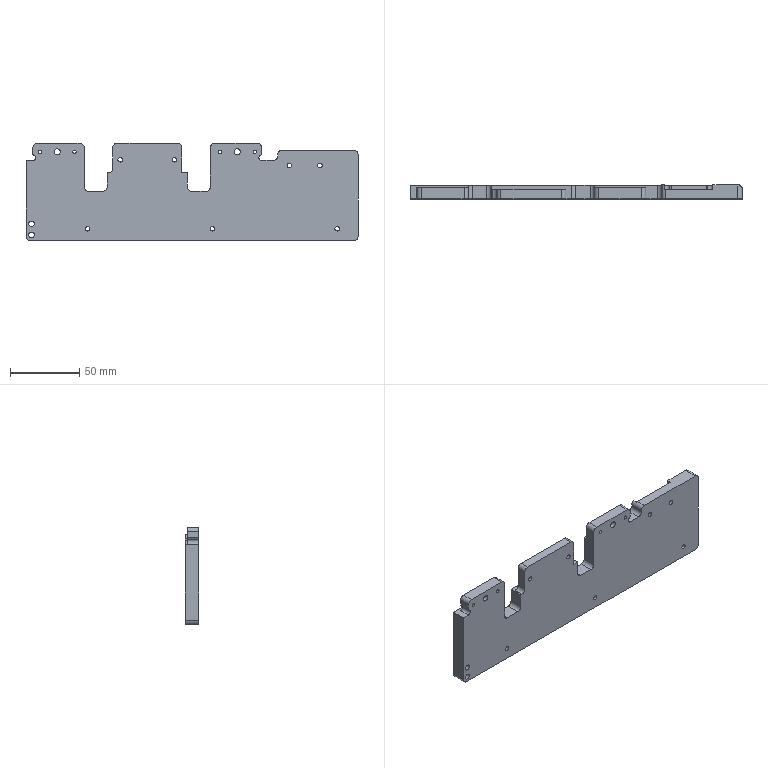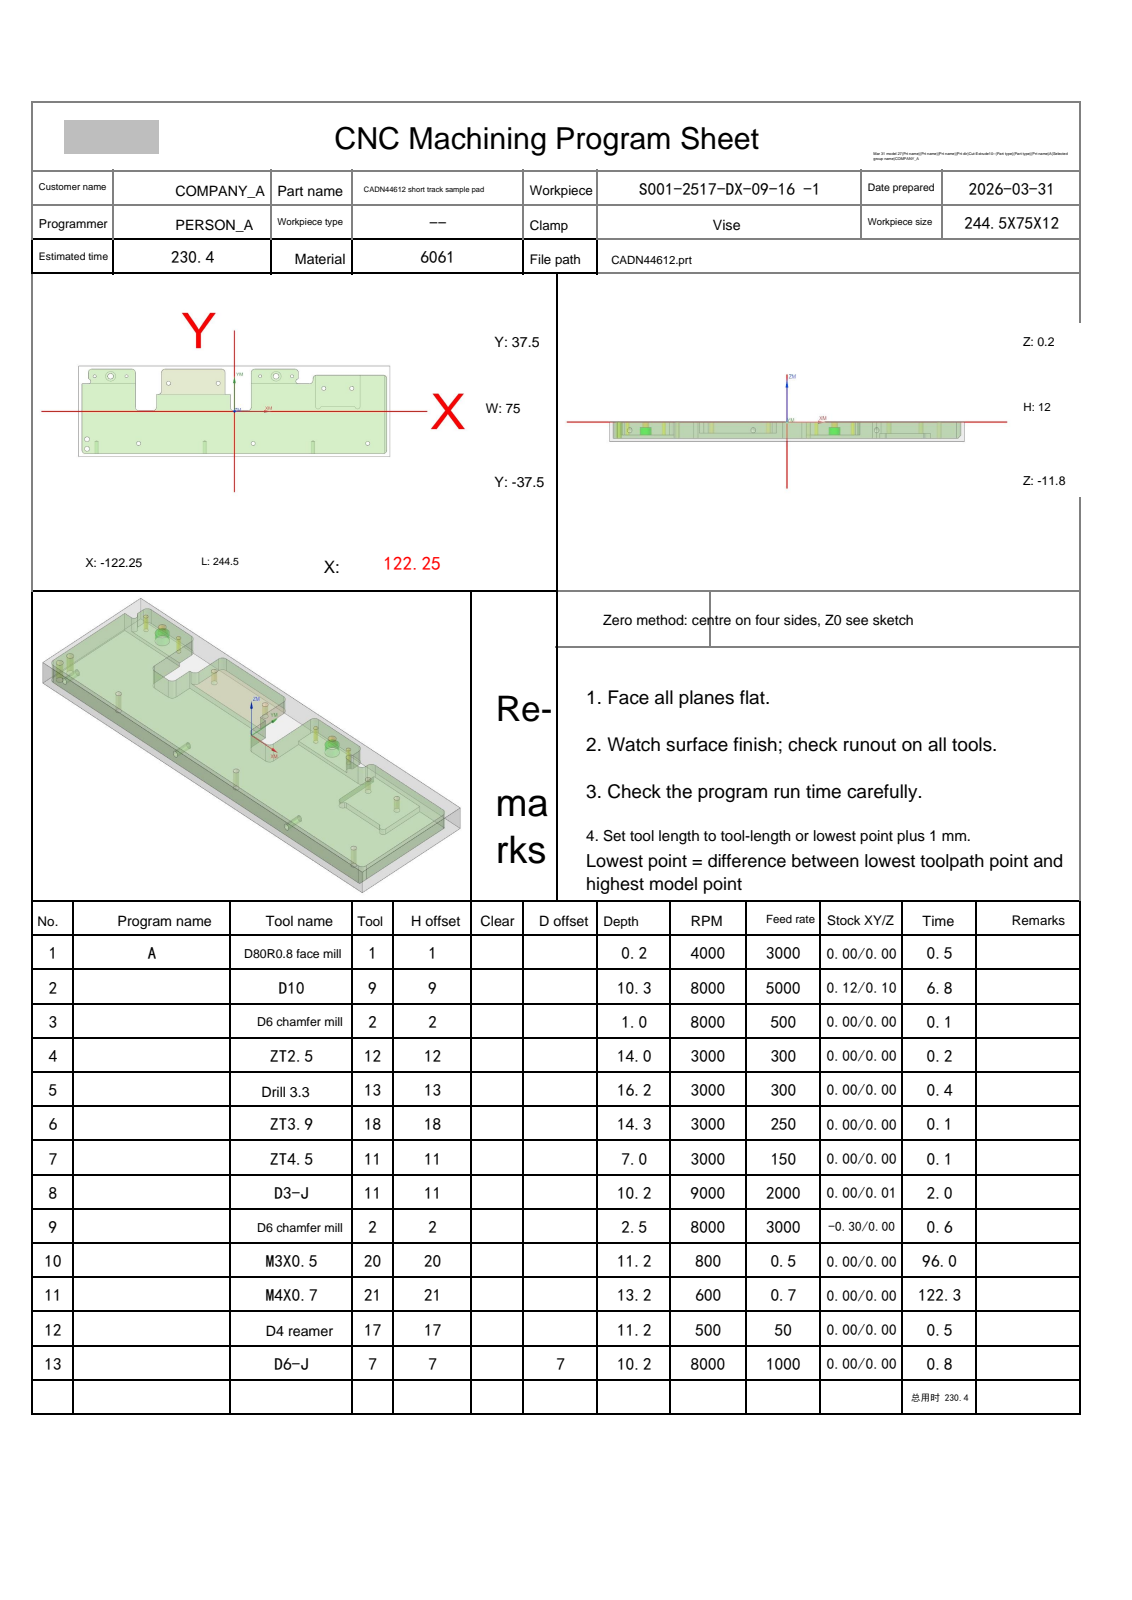NC program | NX | posted by the shop | part box 239.5 x 10 x 70 mm
Lines 2414 to 3395 of 10745:
N8 T11 M06
(D3-J  D=3. R=0. H=11 ce=0.00 di=0.01)
G00 G90 G54 X-120.212 Y24.718 M03 S9000
G43 H11 Z20.
M08
Z.157
G01 X-120.211 Y24.713 Z.093 F1600.
X-120.207 Y24.699 Z.035
X-120.201 Y24.677 Z-.018
X-120.193 Y24.649 Z-.065
X-120.182 Y24.616 Z-.107
X-120.168 Y24.579 Z-.143
X-120.152 Y24.539 Z-.175
X-120.133 Y24.499 Z-.203
X-120.111 Y24.459 Z-.226
X-120.087 Y24.42 Z-.245
X-120.059 Y24.384 Z-.261
X-120.029 Y24.352 Z-.273
X-119.995 Y24.326 Z-.282
X-119.958 Y24.307 Z-.288
X-119.918 Y24.296 Z-.292
X-119.875 Y24.295 Z-.293
X-119.75 Y24.3 F2000.
X-114.75
G03 X-114.25 Y24.8 I0.0 J.5
X-114.583 Y25.271 I-.5 J0.0
G02 X-116.25 Y27.628 I.833 J2.357
G01 Y27.973
X-116.266 Y28.001 Z-.294
X-116.312 Y28.005 Z-.296
X-116.384 Y27.986 Z-.3
X-116.48 Y27.947 Z-.306
X-116.596 Y27.889 Z-.312
X-116.729 Y27.815 Z-.32
X-117.029 Y27.625 Z-.339
X-117.224 Y27.491 Z-.351
X-117.539 Y27.259 Z-.372
X-117.999 Y26.878 Z-.405
X-118.437 Y26.464 Z-.439
X-118.844 Y26.024 Z-.473
X-119.214 Y25.564 Z-.506
X-119.436 Y25.25 Z-.527
X-119.562 Y25.056 Z-.539
X-119.739 Y24.759 Z-.558
X-119.808 Y24.627 Z-.565
X-119.86 Y24.513 Z-.572
X-119.895 Y24.42 Z-.578
X-119.91 Y24.35 Z-.582
X-119.904 Y24.307 Z-.584
X-119.875 Y24.295 Z-.585
X-119.75 Y24.3
X-114.75
G03 X-114.25 Y24.8 I0.0 J.5
X-114.583 Y25.271 I-.5 J0.0
G02 X-116.25 Y27.628 I.833 J2.357
G01 Y27.973
X-116.266 Y28.001 Z-.586
X-116.312 Y28.005 Z-.589
X-116.384 Y27.986 Z-.593
X-116.48 Y27.947 Z-.598
X-116.596 Y27.889 Z-.605
X-116.729 Y27.815 Z-.613
X-117.029 Y27.625 Z-.631
X-117.224 Y27.491 Z-.644
X-117.539 Y27.259 Z-.665
X-117.999 Y26.878 Z-.698
X-118.437 Y26.464 Z-.732
X-118.844 Y26.024 Z-.766
X-119.214 Y25.564 Z-.799
X-119.436 Y25.25 Z-.819
X-119.562 Y25.056 Z-.832
X-119.739 Y24.759 Z-.85
X-119.808 Y24.627 Z-.858
X-119.86 Y24.513 Z-.865
X-119.895 Y24.42 Z-.87
X-119.91 Y24.35 Z-.874
X-119.904 Y24.307 Z-.877
X-119.875 Y24.295 Z-.878
X-119.75 Y24.3
X-114.75
G03 X-114.25 Y24.8 I0.0 J.5
X-114.583 Y25.271 I-.5 J0.0
G02 X-116.25 Y27.628 I.833 J2.357
G01 Y27.973
X-116.266 Y28.001 Z-.879
X-116.312 Y28.005 Z-.881
X-116.384 Y27.986 Z-.885
X-116.48 Y27.947 Z-.891
X-116.596 Y27.889 Z-.898
X-116.729 Y27.815 Z-.906
X-117.029 Y27.625 Z-.924
X-117.224 Y27.491 Z-.936
X-117.539 Y27.259 Z-.957
X-117.999 Y26.878 Z-.99
X-118.437 Y26.464 Z-1.024
X-118.844 Y26.024 Z-1.058
X-119.214 Y25.564 Z-1.091
X-119.436 Y25.25 Z-1.112
X-119.562 Y25.056 Z-1.124
X-119.739 Y24.759 Z-1.143
X-119.808 Y24.627 Z-1.151
X-119.86 Y24.513 Z-1.158
X-119.895 Y24.42 Z-1.163
X-119.91 Y24.35 Z-1.167
X-119.904 Y24.307 Z-1.17
X-119.875 Y24.295 Z-1.171
X-119.75 Y24.3
X-114.75
G03 X-114.25 Y24.8 I0.0 J.5
X-114.583 Y25.271 I-.5 J0.0
G02 X-116.25 Y27.628 I.833 J2.357
G01 Y27.973
X-116.266 Y28.001
X-116.312 Y28.005 Z-1.174
X-116.384 Y27.986 Z-1.178
X-116.48 Y27.947 Z-1.184
X-116.596 Y27.889 Z-1.19
X-116.729 Y27.815 Z-1.198
X-117.029 Y27.625 Z-1.217
X-117.224 Y27.491 Z-1.229
X-117.539 Y27.259 Z-1.25
X-117.999 Y26.878 Z-1.283
X-118.437 Y26.464 Z-1.317
X-118.844 Y26.024 Z-1.351
X-119.214 Y25.564 Z-1.384
X-119.436 Y25.25 Z-1.405
X-119.562 Y25.056 Z-1.417
X-119.739 Y24.759 Z-1.436
X-119.808 Y24.627 Z-1.443
X-119.86 Y24.513 Z-1.45
X-119.895 Y24.42 Z-1.456
X-119.91 Y24.35 Z-1.46
X-119.904 Y24.307 Z-1.462
X-119.875 Y24.295 Z-1.463
X-119.75 Y24.3
X-114.75
G03 X-114.25 Y24.8 I0.0 J.5
X-114.583 Y25.271 I-.5 J0.0
G02 X-116.25 Y27.628 I.833 J2.357
G01 Y27.973
X-116.266 Y28.001 Z-1.464
X-116.312 Y28.005 Z-1.467
X-116.384 Y27.986 Z-1.471
X-116.48 Y27.947 Z-1.476
X-116.596 Y27.889 Z-1.483
X-116.729 Y27.815 Z-1.491
X-117.029 Y27.625 Z-1.509
X-117.224 Y27.491 Z-1.522
X-117.539 Y27.259 Z-1.542
X-117.999 Y26.878 Z-1.575
X-118.437 Y26.464 Z-1.61
X-118.844 Y26.024 Z-1.644
X-119.214 Y25.564 Z-1.677
X-119.436 Y25.25 Z-1.697
X-119.562 Y25.056 Z-1.71
X-119.739 Y24.759 Z-1.728
X-119.808 Y24.627 Z-1.736
X-119.86 Y24.513 Z-1.743
X-119.895 Y24.42 Z-1.748
X-119.91 Y24.35 Z-1.752
X-119.904 Y24.307 Z-1.755
X-119.875 Y24.295 Z-1.756
X-119.75 Y24.3
X-114.75
G03 X-114.25 Y24.8 I0.0 J.5
X-114.583 Y25.271 I-.5 J0.0
G02 X-116.25 Y27.628 I.833 J2.357
G01 Y27.973
X-116.266 Y28.001 Z-1.757
X-116.312 Y28.005 Z-1.759
X-116.384 Y27.986 Z-1.763
X-116.48 Y27.947 Z-1.769
X-116.596 Y27.889 Z-1.776
X-116.729 Y27.815 Z-1.784
X-117.029 Y27.625 Z-1.802
X-117.224 Y27.491 Z-1.814
X-117.539 Y27.259 Z-1.835
X-117.999 Y26.878 Z-1.868
X-118.437 Y26.464 Z-1.902
X-118.844 Y26.024 Z-1.936
X-119.214 Y25.564 Z-1.969
X-119.436 Y25.25 Z-1.99
X-119.562 Y25.056 Z-2.002
X-119.739 Y24.759 Z-2.021
X-119.808 Y24.627 Z-2.029
X-119.86 Y24.513 Z-2.035
X-119.895 Y24.42 Z-2.041
X-119.91 Y24.35 Z-2.045
X-119.904 Y24.307 Z-2.048
X-119.875 Y24.295 Z-2.049
X-119.75 Y24.3
X-114.75
G03 X-114.25 Y24.8 I0.0 J.5
X-114.583 Y25.271 I-.5 J0.0
G02 X-116.25 Y27.628 I.833 J2.357
G01 Y27.973
X-116.266 Y28.001
X-116.312 Y28.005 Z-2.052
X-116.384 Y27.986 Z-2.056
X-116.48 Y27.947 Z-2.062
X-116.596 Y27.889 Z-2.068
X-116.729 Y27.815 Z-2.076
X-117.029 Y27.625 Z-2.095
X-117.224 Y27.491 Z-2.107
X-117.539 Y27.259 Z-2.128
X-117.999 Y26.878 Z-2.161
X-118.437 Y26.464 Z-2.195
X-118.844 Y26.024 Z-2.229
X-119.214 Y25.564 Z-2.262
X-119.436 Y25.25 Z-2.283
X-119.562 Y25.056 Z-2.295
X-119.739 Y24.759 Z-2.313
X-119.808 Y24.627 Z-2.321
X-119.86 Y24.513 Z-2.328
X-119.895 Y24.42 Z-2.334
X-119.91 Y24.35 Z-2.338
X-119.904 Y24.307 Z-2.34
X-119.875 Y24.295 Z-2.341
X-119.75 Y24.3
X-114.75
G03 X-114.25 Y24.8 I0.0 J.5
X-114.583 Y25.271 I-.5 J0.0
G02 X-116.25 Y27.628 I.833 J2.357
G01 Y27.973
X-116.266 Y28.001 Z-2.342
X-116.312 Y28.005 Z-2.345
X-116.384 Y27.986 Z-2.349
X-116.48 Y27.947 Z-2.354
X-116.596 Y27.889 Z-2.361
X-116.729 Y27.815 Z-2.369
X-117.029 Y27.625 Z-2.387
X-117.224 Y27.491 Z-2.4
X-117.539 Y27.259 Z-2.42
X-117.999 Y26.878 Z-2.453
X-118.437 Y26.464 Z-2.488
X-118.844 Y26.024 Z-2.522
X-119.214 Y25.564 Z-2.555
X-119.436 Y25.25 Z-2.575
X-119.562 Y25.056 Z-2.588
X-119.739 Y24.759 Z-2.606
X-119.808 Y24.627 Z-2.614
X-119.86 Y24.513 Z-2.621
X-119.895 Y24.42 Z-2.626
X-119.91 Y24.35 Z-2.63
X-119.904 Y24.307 Z-2.633
X-119.875 Y24.295 Z-2.634
X-119.75 Y24.3
X-114.75
G03 X-114.25 Y24.8 I0.0 J.5
X-114.583 Y25.271 I-.5 J0.0
G02 X-116.25 Y27.628 I.833 J2.357
G01 Y27.973
X-116.266 Y28.001 Z-2.635
X-116.312 Y28.005 Z-2.637
X-116.384 Y27.986 Z-2.641
X-116.48 Y27.947 Z-2.647
X-116.596 Y27.889 Z-2.654
X-116.729 Y27.815 Z-2.662
X-117.029 Y27.625 Z-2.68
X-117.224 Y27.491 Z-2.692
X-117.539 Y27.259 Z-2.713
X-117.999 Y26.878 Z-2.746
X-118.437 Y26.464 Z-2.78
X-118.844 Y26.024 Z-2.814
X-119.214 Y25.564 Z-2.847
X-119.436 Y25.25 Z-2.868
X-119.562 Y25.056 Z-2.88
X-119.739 Y24.759 Z-2.899
X-119.808 Y24.627 Z-2.907
X-119.86 Y24.513 Z-2.913
X-119.895 Y24.42 Z-2.919
X-119.91 Y24.35 Z-2.923
X-119.904 Y24.307 Z-2.926
X-119.875 Y24.295
X-119.75 Y24.3
X-114.75
G03 X-114.25 Y24.8 I0.0 J.5
X-114.583 Y25.271 I-.5 J0.0
G02 X-116.25 Y27.628 I.833 J2.357
G01 Y27.973
X-116.266 Y28.001 Z-2.927
X-116.312 Y28.005 Z-2.93
X-116.384 Y27.986 Z-2.934
X-116.48 Y27.947 Z-2.94
X-116.596 Y27.889 Z-2.946
X-116.729 Y27.815 Z-2.954
X-117.029 Y27.625 Z-2.973
X-117.224 Y27.491 Z-2.985
X-117.539 Y27.259 Z-3.006
X-117.999 Y26.878 Z-3.039
X-118.437 Y26.464 Z-3.073
X-118.844 Y26.024 Z-3.107
X-119.214 Y25.564 Z-3.14
X-119.436 Y25.25 Z-3.161
X-119.562 Y25.056 Z-3.173
X-119.739 Y24.759 Z-3.191
X-119.808 Y24.627 Z-3.199
X-119.86 Y24.513 Z-3.206
X-119.895 Y24.42 Z-3.212
X-119.91 Y24.35 Z-3.216
X-119.904 Y24.307 Z-3.218
X-119.875 Y24.295 Z-3.219
X-119.75 Y24.3
X-114.75
G03 X-114.25 Y24.8 I0.0 J.5
X-114.583 Y25.271 I-.5 J0.0
G02 X-116.25 Y27.628 I.833 J2.357
G01 Y27.973
X-116.266 Y28.001 Z-3.22
X-116.312 Y28.005 Z-3.223
X-116.384 Y27.986 Z-3.227
X-116.48 Y27.947 Z-3.232
X-116.596 Y27.889 Z-3.239
X-116.729 Y27.815 Z-3.247
X-117.029 Y27.625 Z-3.265
X-117.224 Y27.491 Z-3.278
X-117.539 Y27.259 Z-3.298
X-117.999 Y26.878 Z-3.331
X-118.437 Y26.464 Z-3.365
X-118.844 Y26.024 Z-3.4
X-119.214 Y25.564 Z-3.433
X-119.436 Y25.25 Z-3.453
X-119.562 Y25.056 Z-3.466
X-119.739 Y24.759 Z-3.484
X-119.808 Y24.627 Z-3.492
X-119.86 Y24.513 Z-3.499
X-119.895 Y24.42 Z-3.504
X-119.91 Y24.35 Z-3.508
X-119.904 Y24.307 Z-3.511
X-119.875 Y24.295 Z-3.512
X-119.75 Y24.3
X-114.75
G03 X-114.25 Y24.8 I0.0 J.5
X-114.583 Y25.271 I-.5 J0.0
G02 X-116.25 Y27.628 I.833 J2.357
G01 Y27.973
X-116.266 Y28.001 Z-3.513
X-116.312 Y28.005 Z-3.515
X-116.384 Y27.986 Z-3.519
X-116.48 Y27.947 Z-3.525
X-116.596 Y27.889 Z-3.532
X-116.729 Y27.815 Z-3.539
X-117.029 Y27.625 Z-3.558
X-117.224 Y27.491 Z-3.57
X-117.539 Y27.259 Z-3.591
X-117.999 Y26.878 Z-3.624
X-118.437 Y26.464 Z-3.658
X-118.844 Y26.024 Z-3.692
X-119.214 Y25.564 Z-3.725
X-119.436 Y25.25 Z-3.746
X-119.562 Y25.056 Z-3.758
X-119.739 Y24.759 Z-3.777
X-119.808 Y24.627 Z-3.785
X-119.86 Y24.513 Z-3.791
X-119.895 Y24.42 Z-3.797
X-119.91 Y24.35 Z-3.801
X-119.904 Y24.307 Z-3.804
X-119.875 Y24.295
X-119.75 Y24.3
X-114.75
G03 X-114.25 Y24.8 I0.0 J.5
X-114.583 Y25.271 I-.5 J0.0
G02 X-116.25 Y27.628 I.833 J2.357
G01 Y27.973
X-116.266 Y28.001 Z-3.805
X-116.312 Y28.005 Z-3.808
X-116.384 Y27.986 Z-3.812
X-116.48 Y27.947 Z-3.817
X-116.596 Y27.889 Z-3.824
X-116.729 Y27.815 Z-3.832
X-117.029 Y27.625 Z-3.85
X-117.224 Y27.491 Z-3.863
X-117.539 Y27.259 Z-3.884
X-117.999 Y26.878 Z-3.917
X-118.437 Y26.464 Z-3.951
X-118.844 Y26.024 Z-3.985
X-119.214 Y25.564 Z-4.018
X-119.436 Y25.25 Z-4.039
X-119.562 Y25.056 Z-4.051
X-119.739 Y24.759 Z-4.069
X-119.808 Y24.627 Z-4.077
X-119.86 Y24.513 Z-4.084
X-119.895 Y24.42 Z-4.09
X-119.91 Y24.35 Z-4.094
X-119.904 Y24.307 Z-4.096
X-119.875 Y24.295 Z-4.097
X-119.75 Y24.3
X-114.75
G03 X-114.25 Y24.8 I0.0 J.5
X-114.583 Y25.271 I-.5 J0.0
G02 X-116.25 Y27.628 I.833 J2.357
G01 Y27.973
X-116.266 Y28.001 Z-4.098
X-116.312 Y28.005 Z-4.101
X-116.384 Y27.986 Z-4.105
X-116.48 Y27.947 Z-4.11
X-116.596 Y27.889 Z-4.117
X-116.729 Y27.815 Z-4.125
X-117.029 Y27.625 Z-4.143
X-117.224 Y27.491 Z-4.155
X-117.539 Y27.259 Z-4.176
X-117.999 Y26.878 Z-4.209
X-118.437 Y26.464 Z-4.243
X-118.844 Y26.024 Z-4.277
X-119.214 Y25.564 Z-4.31
X-119.436 Y25.25 Z-4.331
X-119.562 Y25.056 Z-4.344
X-119.739 Y24.759 Z-4.362
X-119.808 Y24.627 Z-4.37
X-119.86 Y24.513 Z-4.377
X-119.895 Y24.42 Z-4.382
X-119.91 Y24.35 Z-4.386
X-119.904 Y24.307 Z-4.389
X-119.875 Y24.295 Z-4.39
X-119.75 Y24.3
X-114.75
G03 X-114.25 Y24.8 I0.0 J.5
X-114.583 Y25.271 I-.5 J0.0
G02 X-116.25 Y27.628 I.833 J2.357
G01 Y27.973
X-116.266 Y28.001 Z-4.391
X-116.312 Y28.005 Z-4.393
X-116.384 Y27.986 Z-4.397
X-116.48 Y27.947 Z-4.403
X-116.596 Y27.889 Z-4.41
X-116.729 Y27.815 Z-4.417
X-117.029 Y27.625 Z-4.436
X-117.224 Y27.491 Z-4.448
X-117.539 Y27.259 Z-4.469
X-117.999 Y26.878 Z-4.502
X-118.437 Y26.464 Z-4.536
X-118.844 Y26.024 Z-4.57
X-119.214 Y25.564 Z-4.603
X-119.436 Y25.25 Z-4.624
X-119.562 Y25.056 Z-4.636
X-119.739 Y24.759 Z-4.655
X-119.808 Y24.627 Z-4.663
X-119.86 Y24.513 Z-4.669
X-119.895 Y24.42 Z-4.675
X-119.91 Y24.35 Z-4.679
X-119.904 Y24.307 Z-4.681
X-119.875 Y24.295 Z-4.682
X-119.75 Y24.3
X-114.75
G03 X-114.25 Y24.8 I0.0 J.5
X-114.583 Y25.271 I-.5 J0.0
G02 X-116.25 Y27.628 I.833 J2.357
G01 Y27.973
X-116.266 Y28.001 Z-4.683
X-116.312 Y28.005 Z-4.686
X-116.384 Y27.986 Z-4.69
X-116.48 Y27.947 Z-4.695
X-116.596 Y27.889 Z-4.702
X-116.729 Y27.815 Z-4.71
X-117.029 Y27.625 Z-4.728
X-117.224 Y27.491 Z-4.741
X-117.539 Y27.259 Z-4.762
X-117.999 Y26.878 Z-4.795
X-118.437 Y26.464 Z-4.829
X-118.844 Y26.024 Z-4.863
X-119.214 Y25.564 Z-4.896
X-119.436 Y25.25 Z-4.917
X-119.562 Y25.056 Z-4.929
X-119.739 Y24.759 Z-4.947
X-119.808 Y24.627 Z-4.955
X-119.86 Y24.513 Z-4.962
X-119.895 Y24.42 Z-4.967
X-119.91 Y24.35 Z-4.972
X-119.904 Y24.307 Z-4.974
X-119.875 Y24.295 Z-4.975
X-119.75 Y24.3
X-114.75
G03 X-114.25 Y24.8 I0.0 J.5
X-114.583 Y25.271 I-.5 J0.0
G02 X-116.25 Y27.628 I.833 J2.357
G01 Y27.973
X-116.266 Y28.001 Z-4.976
X-116.312 Y28.005 Z-4.978
X-116.384 Y27.986 Z-4.983
X-116.48 Y27.947 Z-4.988
X-116.596 Y27.889 Z-4.995
X-116.729 Y27.815 Z-5.003
X-117.029 Y27.625 Z-5.021
X-117.224 Y27.491 Z-5.033
X-117.539 Y27.259 Z-5.054
X-117.999 Y26.878 Z-5.087
X-118.437 Y26.464 Z-5.121
X-118.844 Y26.024 Z-5.155
X-119.214 Y25.564 Z-5.188
X-119.436 Y25.25 Z-5.209
X-119.562 Y25.056 Z-5.222
X-119.739 Y24.759 Z-5.24
X-119.808 Y24.627 Z-5.248
X-119.86 Y24.513 Z-5.255
X-119.895 Y24.42 Z-5.26
X-119.91 Y24.35 Z-5.264
X-119.904 Y24.307 Z-5.267
X-119.875 Y24.295 Z-5.268
X-119.75 Y24.3
X-114.75
G03 X-114.25 Y24.8 I0.0 J.5
X-114.583 Y25.271 I-.5 J0.0
G02 X-116.25 Y27.628 I.833 J2.357
G01 Y27.973
X-116.266 Y28.001 Z-5.269
X-116.312 Y28.005 Z-5.271
X-116.384 Y27.986 Z-5.275
X-116.48 Y27.947 Z-5.281
X-116.596 Y27.889 Z-5.287
X-116.729 Y27.815 Z-5.295
X-117.029 Y27.625 Z-5.314
X-117.224 Y27.491 Z-5.326
X-117.539 Y27.259 Z-5.347
X-117.999 Y26.878 Z-5.38
X-118.437 Y26.464 Z-5.414
X-118.844 Y26.024 Z-5.448
X-119.214 Y25.564 Z-5.481
X-119.436 Y25.25 Z-5.502
X-119.562 Y25.056 Z-5.514
X-119.739 Y24.759 Z-5.533
X-119.808 Y24.627 Z-5.54
X-119.86 Y24.513 Z-5.547
X-119.895 Y24.42 Z-5.553
X-119.91 Y24.35 Z-5.557
X-119.904 Y24.307 Z-5.559
X-119.875 Y24.295 Z-5.56
X-119.75 Y24.3
X-114.75
G03 X-114.25 Y24.8 I0.0 J.5
X-114.583 Y25.271 I-.5 J0.0
G02 X-116.25 Y27.628 I.833 J2.357
G01 Y27.973
X-116.266 Y28.001 Z-5.561
X-116.312 Y28.005 Z-5.564
X-116.384 Y27.986 Z-5.568
X-116.48 Y27.947 Z-5.573
X-116.596 Y27.889 Z-5.58
X-116.729 Y27.815 Z-5.588
X-117.029 Y27.625 Z-5.606
X-117.224 Y27.491 Z-5.619
X-117.539 Y27.259 Z-5.64
X-117.999 Y26.878 Z-5.673
X-118.437 Y26.464 Z-5.707
X-118.844 Y26.024 Z-5.741
X-119.214 Y25.564 Z-5.774
X-119.436 Y25.25 Z-5.794
X-119.562 Y25.056 Z-5.807
X-119.739 Y24.759 Z-5.825
X-119.808 Y24.627 Z-5.833
X-119.86 Y24.513 Z-5.84
X-119.895 Y24.42 Z-5.845
X-119.91 Y24.35 Z-5.849
X-119.904 Y24.307 Z-5.852
X-119.875 Y24.295 Z-5.853
X-119.75 Y24.3
X-114.75
G03 X-114.25 Y24.8 I0.0 J.5
X-114.583 Y25.271 I-.5 J0.0
G02 X-116.25 Y27.628 I.833 J2.357
G01 Y27.973
X-116.266 Y28.001 Z-5.854
X-116.312 Y28.005 Z-5.856
X-116.384 Y27.986 Z-5.86
X-116.48 Y27.947 Z-5.866
X-116.596 Y27.889 Z-5.873
X-116.729 Y27.815 Z-5.881
X-117.029 Y27.625 Z-5.899
X-117.224 Y27.491 Z-5.911
X-117.539 Y27.259 Z-5.932
X-117.999 Y26.878 Z-5.965
X-118.437 Y26.464 Z-5.999
X-118.844 Y26.024 Z-6.033
X-119.214 Y25.564 Z-6.066
X-119.436 Y25.25 Z-6.087
X-119.562 Y25.056 Z-6.099
X-119.739 Y24.759 Z-6.118
X-119.808 Y24.627 Z-6.126
X-119.86 Y24.513 Z-6.133
X-119.895 Y24.42 Z-6.138
X-119.91 Y24.35 Z-6.142
X-119.904 Y24.307 Z-6.145
X-119.875 Y24.295 Z-6.146
X-119.75 Y24.3
X-114.75
G03 X-114.25 Y24.8 I0.0 J.5
X-114.583 Y25.271 I-.5 J0.0
G02 X-116.25 Y27.628 I.833 J2.357
G01 Y27.973
X-116.266 Y28.001
X-116.312 Y28.005 Z-6.149
X-116.384 Y27.986 Z-6.153
X-116.48 Y27.947 Z-6.159
X-116.596 Y27.889 Z-6.165
X-116.729 Y27.815 Z-6.173
X-117.029 Y27.625 Z-6.192
X-117.224 Y27.491 Z-6.204
X-117.539 Y27.259 Z-6.225
X-117.999 Y26.878 Z-6.258
X-118.437 Y26.464 Z-6.292
X-118.844 Y26.024 Z-6.326
X-119.214 Y25.564 Z-6.359
X-119.436 Y25.25 Z-6.38
X-119.562 Y25.056 Z-6.392
X-119.739 Y24.759 Z-6.411
X-119.808 Y24.627 Z-6.418
X-119.86 Y24.513 Z-6.425
X-119.895 Y24.42 Z-6.431
X-119.91 Y24.35 Z-6.435
X-119.904 Y24.307 Z-6.437
X-119.875 Y24.295 Z-6.438
X-119.75 Y24.3
X-114.75
G03 X-114.25 Y24.8 I0.0 J.5
X-114.583 Y25.271 I-.5 J0.0
G02 X-116.25 Y27.628 I.833 J2.357
G01 Y27.973
X-116.266 Y28.001 Z-6.439
X-116.312 Y28.005 Z-6.442
X-116.384 Y27.986 Z-6.446
X-116.48 Y27.947 Z-6.451
X-116.596 Y27.889 Z-6.458
X-116.729 Y27.815 Z-6.466
X-117.029 Y27.625 Z-6.484
X-117.224 Y27.491 Z-6.497
X-117.539 Y27.259 Z-6.517
X-117.999 Y26.878 Z-6.55
X-118.437 Y26.464 Z-6.585
X-118.844 Y26.024 Z-6.619
X-119.214 Y25.564 Z-6.652
X-119.436 Y25.25 Z-6.672
X-119.562 Y25.056 Z-6.685
X-119.739 Y24.759 Z-6.703
X-119.808 Y24.627 Z-6.711
X-119.86 Y24.513 Z-6.718
X-119.895 Y24.42 Z-6.723
X-119.91 Y24.35 Z-6.727
X-119.904 Y24.307 Z-6.73
X-119.875 Y24.295 Z-6.731
X-119.75 Y24.3
X-114.75
G03 X-114.25 Y24.8 I0.0 J.5
X-114.583 Y25.271 I-.5 J0.0
G02 X-116.25 Y27.628 I.833 J2.357
G01 Y27.973
X-116.266 Y28.001 Z-6.732
X-116.312 Y28.005 Z-6.734
X-116.384 Y27.986 Z-6.738
X-116.48 Y27.947 Z-6.744
X-116.596 Y27.889 Z-6.751
X-116.729 Y27.815 Z-6.759
X-117.029 Y27.625 Z-6.777
X-117.224 Y27.491 Z-6.789
X-117.539 Y27.259 Z-6.81
X-117.999 Y26.878 Z-6.843
X-118.437 Y26.464 Z-6.877
X-118.844 Y26.024 Z-6.911
X-119.214 Y25.564 Z-6.944
X-119.436 Y25.25 Z-6.965
X-119.562 Y25.056 Z-6.977
X-119.739 Y24.759 Z-6.996
X-119.808 Y24.627 Z-7.004
X-119.86 Y24.513 Z-7.01
X-119.895 Y24.42 Z-7.016
X-119.91 Y24.35 Z-7.02
X-119.904 Y24.307 Z-7.023
X-119.875 Y24.295 Z-7.024
X-119.75 Y24.3
X-114.75
G03 X-114.25 Y24.8 I0.0 J.5
X-114.583 Y25.271 I-.5 J0.0
G02 X-116.25 Y27.628 I.833 J2.357
G01 Y27.973
X-116.266 Y28.001
X-116.312 Y28.005 Z-7.027
X-116.384 Y27.986 Z-7.031
X-116.48 Y27.947 Z-7.037
X-116.596 Y27.889 Z-7.043
X-116.729 Y27.815 Z-7.051
X-117.029 Y27.625 Z-7.07
X-117.224 Y27.491 Z-7.082
X-117.539 Y27.259 Z-7.103
X-117.999 Y26.878 Z-7.136
X-118.437 Y26.464 Z-7.17
X-118.844 Y26.024 Z-7.204
X-119.214 Y25.564 Z-7.237
X-119.436 Y25.25 Z-7.258
X-119.562 Y25.056 Z-7.27
X-119.739 Y24.759 Z-7.288
X-119.808 Y24.627 Z-7.296
X-119.86 Y24.513 Z-7.303
X-119.895 Y24.42 Z-7.309
X-119.91 Y24.35 Z-7.313
X-119.904 Y24.307 Z-7.315
X-119.875 Y24.295 Z-7.316
X-119.75 Y24.3
X-114.75
G03 X-114.25 Y24.8 I0.0 J.5
X-114.583 Y25.271 I-.5 J0.0
G02 X-116.25 Y27.628 I.833 J2.357
G01 Y27.973
X-116.266 Y28.001 Z-7.317
X-116.312 Y28.005 Z-7.32
X-116.384 Y27.986 Z-7.324
X-116.48 Y27.947 Z-7.329
X-116.596 Y27.889 Z-7.336
X-116.729 Y27.815 Z-7.344
X-117.029 Y27.625 Z-7.362
X-117.224 Y27.491 Z-7.375
X-117.539 Y27.259 Z-7.395
X-117.999 Y26.878 Z-7.428
X-118.437 Y26.464 Z-7.463
X-118.844 Y26.024 Z-7.497
X-119.214 Y25.564 Z-7.53
X-119.436 Y25.25 Z-7.55
X-119.562 Y25.056 Z-7.563
X-119.739 Y24.759 Z-7.581
X-119.808 Y24.627 Z-7.589
X-119.86 Y24.513 Z-7.596
X-119.895 Y24.42 Z-7.601
X-119.91 Y24.35 Z-7.605
X-119.904 Y24.307 Z-7.608
X-119.875 Y24.295 Z-7.609
X-119.75 Y24.3
X-114.75
G03 X-114.25 Y24.8 I0.0 J.5
X-114.583 Y25.271 I-.5 J0.0
G02 X-116.25 Y27.628 I.833 J2.357
G01 Y27.973
X-116.266 Y28.001 Z-7.61
X-116.312 Y28.005 Z-7.612
X-116.384 Y27.986 Z-7.616
X-116.48 Y27.947 Z-7.622
X-116.596 Y27.889 Z-7.629
X-116.729 Y27.815 Z-7.637
X-117.029 Y27.625 Z-7.655
X-117.224 Y27.491 Z-7.667
X-117.539 Y27.259 Z-7.688
X-117.999 Y26.878 Z-7.721
X-118.437 Y26.464 Z-7.755
X-118.844 Y26.024 Z-7.789
X-119.214 Y25.564 Z-7.822
X-119.436 Y25.25 Z-7.843
X-119.562 Y25.056 Z-7.855
X-119.739 Y24.759 Z-7.874
X-119.808 Y24.627 Z-7.882
X-119.86 Y24.513 Z-7.888
X-119.895 Y24.42 Z-7.894
X-119.91 Y24.35 Z-7.898
X-119.904 Y24.307 Z-7.901
X-119.875 Y24.295
X-119.75 Y24.3
X-114.75
G03 X-114.25 Y24.8 I0.0 J.5
X-114.583 Y25.271 I-.5 J0.0
G02 X-116.25 Y27.628 I.833 J2.357
G01 Y27.973
X-116.266 Y28.001 Z-7.902
X-116.312 Y28.005 Z-7.905
X-116.384 Y27.986 Z-7.909
X-116.48 Y27.947 Z-7.915
X-116.596 Y27.889 Z-7.921
X-116.729 Y27.815 Z-7.929
X-117.029 Y27.625 Z-7.948
X-117.224 Y27.491 Z-7.96
X-117.539 Y27.259 Z-7.981
X-117.999 Y26.878 Z-8.014
X-118.437 Y26.464 Z-8.048
X-118.844 Y26.024 Z-8.082
X-119.214 Y25.564 Z-8.115
X-119.436 Y25.25 Z-8.136
X-119.562 Y25.056 Z-8.148
X-119.739 Y24.759 Z-8.166
X-119.808 Y24.627 Z-8.174
X-119.86 Y24.513 Z-8.181
X-119.895 Y24.42 Z-8.187
X-119.91 Y24.35 Z-8.191
X-119.904 Y24.307 Z-8.193
X-119.875 Y24.295 Z-8.194
X-119.75 Y24.3
X-114.75
G03 X-114.25 Y24.8 I0.0 J.5
X-114.583 Y25.271 I-.5 J0.0
G02 X-116.25 Y27.628 I.833 J2.357
G01 Y27.973
X-116.266 Y28.001 Z-8.195
X-116.312 Y28.005 Z-8.198
X-116.384 Y27.986 Z-8.202
X-116.48 Y27.947 Z-8.207
X-116.596 Y27.889 Z-8.214
X-116.729 Y27.815 Z-8.222
X-117.029 Y27.625 Z-8.24
X-117.224 Y27.491 Z-8.253
X-117.539 Y27.259 Z-8.273
X-117.999 Y26.878 Z-8.306
X-118.437 Y26.464 Z-8.34
X-118.844 Y26.024 Z-8.375
X-119.214 Y25.564 Z-8.408
X-119.436 Y25.25 Z-8.428
X-119.562 Y25.056 Z-8.441
X-119.739 Y24.759 Z-8.459
X-119.808 Y24.627 Z-8.467
X-119.86 Y24.513 Z-8.474
X-119.895 Y24.42 Z-8.479
X-119.91 Y24.35 Z-8.483
X-119.904 Y24.307 Z-8.486
X-119.875 Y24.295 Z-8.487
X-119.75 Y24.3
X-114.75
G03 X-114.25 Y24.8 I0.0 J.5
X-114.583 Y25.271 I-.5 J0.0
G02 X-116.25 Y27.628 I.833 J2.357
G01 Y27.973
X-116.266 Y28.001 Z-8.488
X-116.312 Y28.005 Z-8.49
X-116.384 Y27.986 Z-8.494
X-116.48 Y27.947 Z-8.5
X-116.596 Y27.889 Z-8.507
X-116.729 Y27.815 Z-8.514
X-117.029 Y27.625 Z-8.533
X-117.224 Y27.491 Z-8.545
X-117.539 Y27.259 Z-8.566
X-117.999 Y26.878 Z-8.599
X-118.437 Y26.464 Z-8.633
X-118.844 Y26.024 Z-8.667
X-119.214 Y25.564 Z-8.7
X-119.436 Y25.25 Z-8.721
X-119.562 Y25.056 Z-8.733
X-119.739 Y24.759 Z-8.752
X-119.808 Y24.627 Z-8.76
X-119.86 Y24.513 Z-8.766
X-119.895 Y24.42 Z-8.772
X-119.91 Y24.35 Z-8.776
X-119.904 Y24.307 Z-8.779
X-119.875 Y24.295
X-119.75 Y24.3
X-114.75
G03 X-114.25 Y24.8 I0.0 J.5
X-114.583 Y25.271 I-.5 J0.0
G02 X-116.25 Y27.628 I.833 J2.357
G01 Y27.973
X-116.266 Y28.001 Z-8.78
X-116.312 Y28.005 Z-8.783
X-116.384 Y27.986 Z-8.787
X-116.48 Y27.947 Z-8.792
X-116.596 Y27.889 Z-8.799
X-116.729 Y27.815 Z-8.807
X-117.029 Y27.625 Z-8.825
X-117.224 Y27.491 Z-8.838
X-117.539 Y27.259 Z-8.859
X-117.999 Y26.878 Z-8.892
X-118.437 Y26.464 Z-8.926
X-118.844 Y26.024 Z-8.96
X-119.214 Y25.564 Z-8.993
X-119.436 Y25.25 Z-9.014
X-119.562 Y25.056 Z-9.026
X-119.739 Y24.759 Z-9.044
X-119.808 Y24.627 Z-9.052
X-119.86 Y24.513 Z-9.059
X-119.895 Y24.42 Z-9.065
X-119.91 Y24.35 Z-9.069
X-119.904 Y24.307 Z-9.071
X-119.875 Y24.295 Z-9.072
X-119.75 Y24.3
X-114.75
G03 X-114.25 Y24.8 I0.0 J.5
X-114.583 Y25.271 I-.5 J0.0
G02 X-116.25 Y27.628 I.833 J2.357
G01 Y27.973
X-116.266 Y28.001 Z-9.073
X-116.312 Y28.005 Z-9.076
X-116.384 Y27.986 Z-9.08
X-116.48 Y27.947 Z-9.085
X-116.596 Y27.889 Z-9.092
X-116.729 Y27.815 Z-9.1
X-117.029 Y27.625 Z-9.118
X-117.224 Y27.491 Z-9.13
X-117.539 Y27.259 Z-9.151
X-117.999 Y26.878 Z-9.184
X-118.437 Y26.464 Z-9.218
X-118.844 Y26.024 Z-9.252
X-119.214 Y25.564 Z-9.285
X-119.436 Y25.25 Z-9.306
X-119.562 Y25.056 Z-9.319
X-119.739 Y24.759 Z-9.337
X-119.808 Y24.627 Z-9.345
X-119.86 Y24.513 Z-9.352
X-119.895 Y24.42 Z-9.357
X-119.91 Y24.35 Z-9.361
X-119.904 Y24.307 Z-9.364
X-119.875 Y24.295 Z-9.365
X-119.75 Y24.3
X-114.75
G03 X-114.25 Y24.8 I0.0 J.5
X-114.583 Y25.271 I-.5 J0.0
G02 X-116.25 Y27.628 I.833 J2.357
G01 Y27.973
X-116.266 Y28.001 Z-9.366
X-116.312 Y28.005 Z-9.368
X-116.384 Y27.986 Z-9.372
X-116.48 Y27.947 Z-9.378
X-116.596 Y27.889 Z-9.385
X-116.729 Y27.815 Z-9.392
X-117.029 Y27.625 Z-9.411
X-117.224 Y27.491 Z-9.423
X-117.539 Y27.259 Z-9.444
X-117.999 Y26.878 Z-9.477
X-118.437 Y26.464 Z-9.511
X-118.844 Y26.024 Z-9.545
X-119.214 Y25.564 Z-9.578
X-119.436 Y25.25 Z-9.599
X-119.562 Y25.056 Z-9.611
X-119.739 Y24.759 Z-9.63
X-119.808 Y24.627 Z-9.638
X-119.86 Y24.513 Z-9.644
X-119.895 Y24.42 Z-9.65
X-119.91 Y24.35 Z-9.654
X-119.904 Y24.307 Z-9.656
X-119.875 Y24.295 Z-9.657
X-119.75 Y24.3
X-114.75
G03 X-114.25 Y24.8 I0.0 J.5
X-114.583 Y25.271 I-.5 J0.0
G02 X-116.25 Y27.628 I.833 J2.357
G01 Y27.973
X-116.266 Y28.001 Z-9.658
X-116.312 Y28.005 Z-9.661
X-116.384 Y27.986 Z-9.665
X-116.48 Y27.947 Z-9.67
X-116.596 Y27.889 Z-9.677
X-116.729 Y27.815 Z-9.685
X-117.029 Y27.625 Z-9.703
X-117.224 Y27.491 Z-9.716
X-117.539 Y27.259 Z-9.737
X-117.999 Y26.878 Z-9.77
X-118.437 Y26.464 Z-9.804
X-118.844 Y26.024 Z-9.838
X-119.214 Y25.564 Z-9.871
X-119.436 Y25.25 Z-9.892
X-119.562 Y25.056 Z-9.904
X-119.739 Y24.759 Z-9.922
X-119.808 Y24.627 Z-9.93
X-119.86 Y24.513 Z-9.937
X-119.895 Y24.42 Z-9.942
X-119.91 Y24.35 Z-9.947
X-119.904 Y24.307 Z-9.949
X-119.875 Y24.295 Z-9.95
X-119.75 Y24.3
X-114.75
G03 X-114.25 Y24.8 I0.0 J.5
X-114.583 Y25.271 I-.5 J0.0
G02 X-116.25 Y27.628 I.833 J2.357
G01 Y27.973
X-116.275 Y28.014 Z-9.949
X-116.309 Y28.05 Z-9.945
X-116.349 Y28.082 Z-9.938
X-116.395 Y28.109 Z-9.927
X-116.445 Y28.133 Z-9.913
X-116.497 Y28.153 Z-9.895
X-116.551 Y28.169 Z-9.873
X-116.603 Y28.183 Z-9.846
X-116.654 Y28.193 Z-9.814
X-116.701 Y28.201 Z-9.777
X-116.743 Y28.207 Z-9.734
X-116.778 Y28.212 Z-9.685
X-116.805 Y28.214 Z-9.63
X-116.822 Y28.216 Z-9.568
X-116.828 Z-9.5
G00 Z20.
X-75.672 Y5.897
Z.157
G01 X-75.679 Y5.896 Z.089 F1600.
X-75.696 Y5.894 Z.027
X-75.723 Y5.89 Z-.028
X-75.758 Y5.884 Z-.076
X-75.8 Y5.875 Z-.119
X-75.847 Y5.864 Z-.157
X-75.897 Y5.851 Z-.189
X-75.95 Y5.834 Z-.216
X-76.003 Y5.815 Z-.238
X-76.055 Y5.792 Z-.256
X-76.105 Y5.767 Z-.27
X-76.151 Y5.737 Z-.28